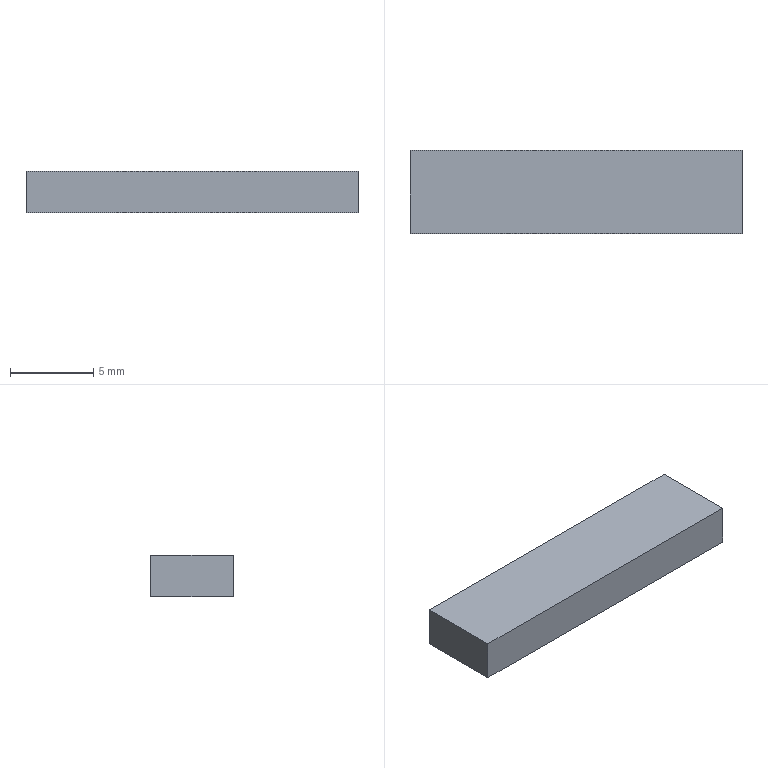Part | STEP file | lll_id1006_x_t | 1 solid | 42 faces | box 20 x 5 x 2.5 mm | volume 247.732 mm3 | other 24 | plane 18